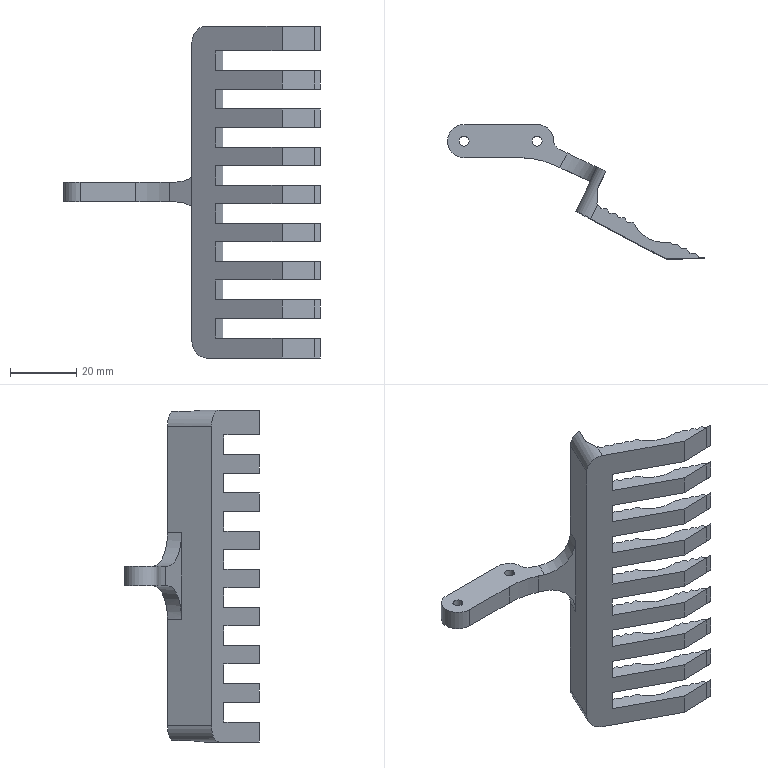Part | SolidWorks | features ICE 7, Fillet 2, Extrusion 1 | 1 solid | 197 faces | box 77.412 x 40.573 x 100 mm | volume 15477 mm3 | plane 176 | cylinder 21 | commonest cylinder face diameters 20 x11 3 x4 10 x4 6 x1 50 x1